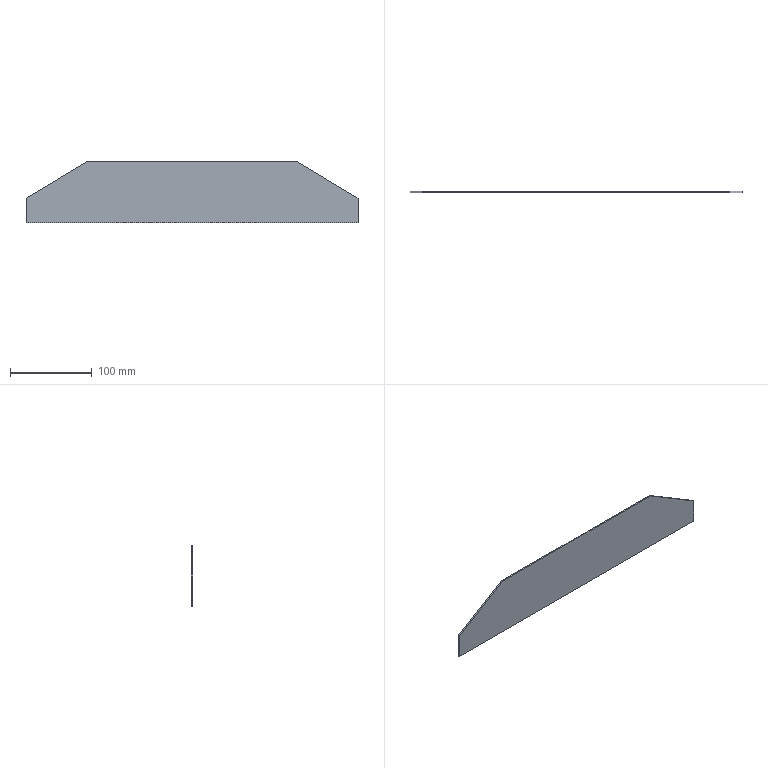Part | SolidWorks | features BaseBody 1 | 1 solid | 8 faces | box 405 x 1.5 x 75 mm | volume 40500 mm3 | plane 8
STEP:
#1=CARTESIAN_POINT('',(202.5,-1.5,-45.));
#2=VERTEX_POINT('',#1);
#3=CARTESIAN_POINT('',(127.5,-1.5,0.));
#4=VERTEX_POINT('',#3);
#5=CARTESIAN_POINT('',(202.5,-1.5,-45.));
#6=DIRECTION('',(-0.8575,0.,0.5145));
#7=VECTOR('',#6,1000.);
#8=LINE('',#5,#7);
#9=EDGE_CURVE('',#2,#4,#8,.T.);
#10=ORIENTED_EDGE('',*,*,#9,.T.);
#11=CARTESIAN_POINT('',(-127.5,-1.5,0.));
#12=VERTEX_POINT('',#11);
#13=CARTESIAN_POINT('',(0.,-1.5,0.));
#14=DIRECTION('',(-1.,0.,0.));
#15=VECTOR('',#14,1000.);
#16=LINE('',#13,#15);
#17=EDGE_CURVE('',#4,#12,#16,.T.);
#18=ORIENTED_EDGE('',*,*,#17,.T.);
#19=CARTESIAN_POINT('',(-202.5,-1.5,-45.));
#20=VERTEX_POINT('',#19);
#21=CARTESIAN_POINT('',(-127.5,-1.5,0.));
#22=DIRECTION('',(-0.8575,0.,-0.5145));
#23=VECTOR('',#22,1000.);
#24=LINE('',#21,#23);
#25=EDGE_CURVE('',#12,#20,#24,.T.);
#26=ORIENTED_EDGE('',*,*,#25,.T.);
#27=CARTESIAN_POINT('',(-202.5,-1.5,-75.));
#28=VERTEX_POINT('',#27);
#29=CARTESIAN_POINT('',(-202.5,-1.5,0.));
#30=DIRECTION('',(0.,0.,-1.));
#31=VECTOR('',#30,1000.);
#32=LINE('',#29,#31);
#33=EDGE_CURVE('',#20,#28,#32,.T.);
#34=ORIENTED_EDGE('',*,*,#33,.T.);
#35=CARTESIAN_POINT('',(202.5,-1.5,-75.));
#36=VERTEX_POINT('',#35);
#37=CARTESIAN_POINT('',(0.,-1.5,-75.));
#38=DIRECTION('',(1.,0.,0.));
#39=VECTOR('',#38,1000.);
#40=LINE('',#37,#39);
#41=EDGE_CURVE('',#28,#36,#40,.T.);
#42=ORIENTED_EDGE('',*,*,#41,.T.);
#43=CARTESIAN_POINT('',(202.5,-1.5,0.));
#44=DIRECTION('',(0.,0.,1.));
#45=VECTOR('',#44,1000.);
#46=LINE('',#43,#45);
#47=EDGE_CURVE('',#36,#2,#46,.T.);
#48=ORIENTED_EDGE('',*,*,#47,.T.);
#49=EDGE_LOOP('',(#10,#18,#26,#34,#42,#48));
#50=FACE_OUTER_BOUND('',#49,.T.);
#51=CARTESIAN_POINT('',(0.,-1.5,0.));
#52=DIRECTION('',(0.,-1.,0.));
#53=DIRECTION('',(0.,0.,-1.));
#54=AXIS2_PLACEMENT_3D('',#51,#52,#53);
#55=PLANE('',#54);
#56=ADVANCED_FACE('',(#50),#55,.T.);
#57=ORIENTED_EDGE('',*,*,#17,.F.);
#58=CARTESIAN_POINT('',(127.5,0.,0.));
#59=VERTEX_POINT('',#58);
#60=CARTESIAN_POINT('',(127.5,-1.5,0.));
#61=DIRECTION('',(0.,1.,0.));
#62=VECTOR('',#61,1000.);
#63=LINE('',#60,#62);
#64=EDGE_CURVE('',#4,#59,#63,.T.);
#65=ORIENTED_EDGE('',*,*,#64,.T.);
#66=CARTESIAN_POINT('',(-127.5,0.,0.));
#67=VERTEX_POINT('',#66);
#68=CARTESIAN_POINT('',(-127.5,0.,0.));
#69=DIRECTION('',(-1.,0.,0.));
#70=VECTOR('',#69,1000.);
#71=LINE('',#68,#70);
#72=EDGE_CURVE('',#59,#67,#71,.T.);
#73=ORIENTED_EDGE('',*,*,#72,.T.);
#74=CARTESIAN_POINT('',(-127.5,-1.5,0.));
#75=DIRECTION('',(0.,-1.,0.));
#76=VECTOR('',#75,1000.);
#77=LINE('',#74,#76);
#78=EDGE_CURVE('',#67,#12,#77,.T.);
#79=ORIENTED_EDGE('',*,*,#78,.T.);
#80=EDGE_LOOP('',(#57,#65,#73,#79));
#81=FACE_OUTER_BOUND('',#80,.T.);
#82=CARTESIAN_POINT('',(-127.5,-1.5,0.));
#83=DIRECTION('',(0.,0.,1.));
#84=DIRECTION('',(1.,0.,0.));
#85=AXIS2_PLACEMENT_3D('',#82,#83,#84);
#86=PLANE('',#85);
#87=ADVANCED_FACE('',(#81),#86,.T.);
#88=ORIENTED_EDGE('',*,*,#9,.F.);
#89=CARTESIAN_POINT('',(202.5,0.,-45.));
#90=VERTEX_POINT('',#89);
#91=CARTESIAN_POINT('',(202.5,-1.5,-45.));
#92=DIRECTION('',(0.,1.,0.));
#93=VECTOR('',#92,1000.);
#94=LINE('',#91,#93);
#95=EDGE_CURVE('',#2,#90,#94,.T.);
#96=ORIENTED_EDGE('',*,*,#95,.T.);
#97=CARTESIAN_POINT('',(127.5,0.,0.));
#98=DIRECTION('',(-0.8575,0.,0.5145));
#99=VECTOR('',#98,1000.);
#100=LINE('',#97,#99);
#101=EDGE_CURVE('',#90,#59,#100,.T.);
#102=ORIENTED_EDGE('',*,*,#101,.T.);
#103=ORIENTED_EDGE('',*,*,#64,.F.);
#104=EDGE_LOOP('',(#88,#96,#102,#103));
#105=FACE_OUTER_BOUND('',#104,.T.);
#106=CARTESIAN_POINT('',(127.5,-1.5,0.));
#107=DIRECTION('',(0.5145,0.,0.8575));
#108=DIRECTION('',(0.8575,0.,-0.5145));
#109=AXIS2_PLACEMENT_3D('',#106,#107,#108);
#110=PLANE('',#109);
#111=ADVANCED_FACE('',(#105),#110,.T.);
#112=ORIENTED_EDGE('',*,*,#47,.F.);
#113=CARTESIAN_POINT('',(202.5,0.,-75.));
#114=VERTEX_POINT('',#113);
#115=CARTESIAN_POINT('',(202.5,-1.5,-75.));
#116=DIRECTION('',(0.,1.,0.));
#117=VECTOR('',#116,1000.);
#118=LINE('',#115,#117);
#119=EDGE_CURVE('',#36,#114,#118,.T.);
#120=ORIENTED_EDGE('',*,*,#119,.T.);
#121=CARTESIAN_POINT('',(202.5,0.,-45.));
#122=DIRECTION('',(0.,0.,1.));
#123=VECTOR('',#122,1000.);
#124=LINE('',#121,#123);
#125=EDGE_CURVE('',#114,#90,#124,.T.);
#126=ORIENTED_EDGE('',*,*,#125,.T.);
#127=ORIENTED_EDGE('',*,*,#95,.F.);
#128=EDGE_LOOP('',(#112,#120,#126,#127));
#129=FACE_OUTER_BOUND('',#128,.T.);
#130=CARTESIAN_POINT('',(202.5,-1.5,-45.));
#131=DIRECTION('',(1.,0.,0.));
#132=DIRECTION('',(0.,0.,-1.));
#133=AXIS2_PLACEMENT_3D('',#130,#131,#132);
#134=PLANE('',#133);
#135=ADVANCED_FACE('',(#129),#134,.T.);
#136=ORIENTED_EDGE('',*,*,#41,.F.);
#137=CARTESIAN_POINT('',(-202.5,0.,-75.));
#138=VERTEX_POINT('',#137);
#139=CARTESIAN_POINT('',(-202.5,-1.5,-75.));
#140=DIRECTION('',(0.,1.,0.));
#141=VECTOR('',#140,1000.);
#142=LINE('',#139,#141);
#143=EDGE_CURVE('',#28,#138,#142,.T.);
#144=ORIENTED_EDGE('',*,*,#143,.T.);
#145=CARTESIAN_POINT('',(-202.5,0.,-75.));
#146=DIRECTION('',(1.,0.,0.));
#147=VECTOR('',#146,1000.);
#148=LINE('',#145,#147);
#149=EDGE_CURVE('',#138,#114,#148,.T.);
#150=ORIENTED_EDGE('',*,*,#149,.T.);
#151=ORIENTED_EDGE('',*,*,#119,.F.);
#152=EDGE_LOOP('',(#136,#144,#150,#151));
#153=FACE_OUTER_BOUND('',#152,.T.);
#154=CARTESIAN_POINT('',(-202.5,-1.5,-75.));
#155=DIRECTION('',(0.,0.,-1.));
#156=DIRECTION('',(-1.,0.,0.));
#157=AXIS2_PLACEMENT_3D('',#154,#155,#156);
#158=PLANE('',#157);
#159=ADVANCED_FACE('',(#153),#158,.T.);
#160=ORIENTED_EDGE('',*,*,#33,.F.);
#161=CARTESIAN_POINT('',(-202.5,0.,-45.));
#162=VERTEX_POINT('',#161);
#163=CARTESIAN_POINT('',(-202.5,-1.5,-45.));
#164=DIRECTION('',(0.,1.,0.));
#165=VECTOR('',#164,1000.);
#166=LINE('',#163,#165);
#167=EDGE_CURVE('',#20,#162,#166,.T.);
#168=ORIENTED_EDGE('',*,*,#167,.T.);
#169=CARTESIAN_POINT('',(-202.5,0.,-45.));
#170=DIRECTION('',(0.,0.,-1.));
#171=VECTOR('',#170,1000.);
#172=LINE('',#169,#171);
#173=EDGE_CURVE('',#162,#138,#172,.T.);
#174=ORIENTED_EDGE('',*,*,#173,.T.);
#175=ORIENTED_EDGE('',*,*,#143,.F.);
#176=EDGE_LOOP('',(#160,#168,#174,#175));
#177=FACE_OUTER_BOUND('',#176,.T.);
#178=CARTESIAN_POINT('',(-202.5,-1.5,-45.));
#179=DIRECTION('',(-1.,0.,0.));
#180=DIRECTION('',(0.,0.,1.));
#181=AXIS2_PLACEMENT_3D('',#178,#179,#180);
#182=PLANE('',#181);
#183=ADVANCED_FACE('',(#177),#182,.T.);
#184=ORIENTED_EDGE('',*,*,#25,.F.);
#185=ORIENTED_EDGE('',*,*,#78,.F.);
#186=CARTESIAN_POINT('',(-127.5,0.,0.));
#187=DIRECTION('',(-0.8575,0.,-0.5145));
#188=VECTOR('',#187,1000.);
#189=LINE('',#186,#188);
#190=EDGE_CURVE('',#67,#162,#189,.T.);
#191=ORIENTED_EDGE('',*,*,#190,.T.);
#192=ORIENTED_EDGE('',*,*,#167,.F.);
#193=EDGE_LOOP('',(#184,#185,#191,#192));
#194=FACE_OUTER_BOUND('',#193,.T.);
#195=CARTESIAN_POINT('',(-127.5,-1.5,0.));
#196=DIRECTION('',(-0.5145,0.,0.8575));
#197=DIRECTION('',(0.8575,0.,0.5145));
#198=AXIS2_PLACEMENT_3D('',#195,#196,#197);
#199=PLANE('',#198);
#200=ADVANCED_FACE('',(#194),#199,.T.);
#201=ORIENTED_EDGE('',*,*,#72,.F.);
#202=ORIENTED_EDGE('',*,*,#101,.F.);
#203=ORIENTED_EDGE('',*,*,#125,.F.);
#204=ORIENTED_EDGE('',*,*,#149,.F.);
#205=ORIENTED_EDGE('',*,*,#173,.F.);
#206=ORIENTED_EDGE('',*,*,#190,.F.);
#207=EDGE_LOOP('',(#201,#202,#203,#204,#205,#206));
#208=FACE_OUTER_BOUND('',#207,.T.);
#209=CARTESIAN_POINT('',(0.,0.,0.));
#210=DIRECTION('',(0.,-1.,0.));
#211=DIRECTION('',(0.,0.,-1.));
#212=AXIS2_PLACEMENT_3D('',#209,#210,#211);
#213=PLANE('',#212);
#214=ADVANCED_FACE('',(#208),#213,.F.);
#215=CLOSED_SHELL('',(#56,#87,#111,#135,#159,#183,#200,#214));
#216=MANIFOLD_SOLID_BREP('',#215);
#217=CARTESIAN_POINT('',(0.,0.,0.));
#218=DIRECTION('',(0.,0.,1.));
#219=DIRECTION('',(1.,0.,0.));
#220=AXIS2_PLACEMENT_3D('',#217,#218,#219);
#221=(LENGTH_UNIT()NAMED_UNIT(*)SI_UNIT(.MILLI.,.METRE.));
#222=UNCERTAINTY_MEASURE_WITH_UNIT(LENGTH_MEASURE(0.00001),#221,'','');
#223=(NAMED_UNIT(*)PLANE_ANGLE_UNIT()SI_UNIT($,.RADIAN.));
#224=(NAMED_UNIT(*)SI_UNIT($,.STERADIAN.)SOLID_ANGLE_UNIT());
#225=(GEOMETRIC_REPRESENTATION_CONTEXT(3)GLOBAL_UNCERTAINTY_ASSIGNED_CONTEXT((#222))GLOBAL_UNIT_ASSIGNED_CONTEXT((#221,#223,#224))REPRESENTATION_CONTEXT('',''));
#226=ADVANCED_BREP_SHAPE_REPRESENTATION('',(#216,#220),#225);